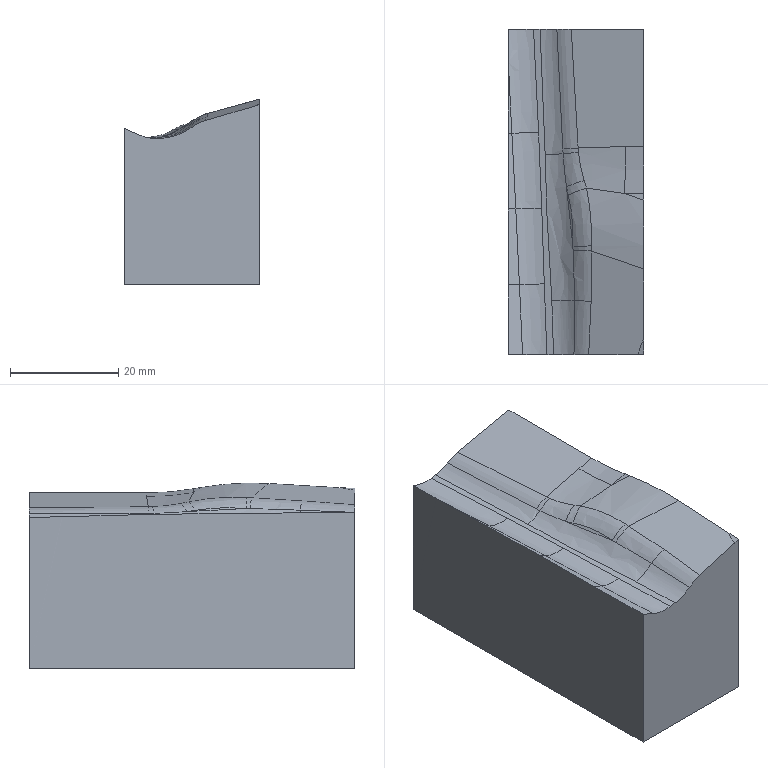Part | NX | features solid 2 | 1 solid | 33 faces | box 25 x 60 x 34.314 mm | volume 44697 mm3 | spline 28 | plane 5